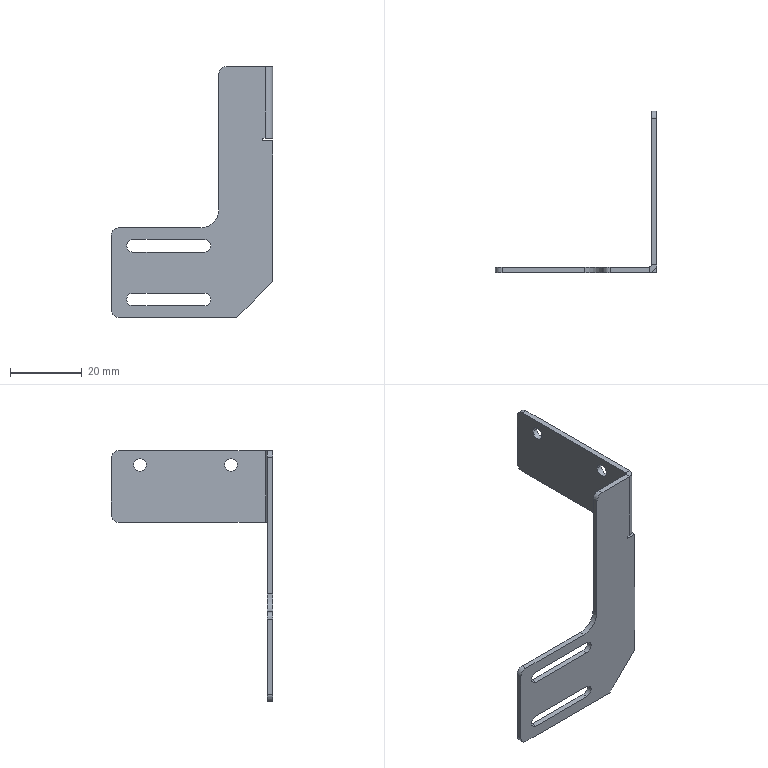Part | STEP file | Sensor Mounting Plate | 1 solid | 39 faces | box 45 x 45 x 70 mm | volume 3643 mm3 | plane 23 | cylinder 16 | commonest cylinder face diameters 3.5 x8 4 x5 1.2 x1 4.2 x1 10 x1